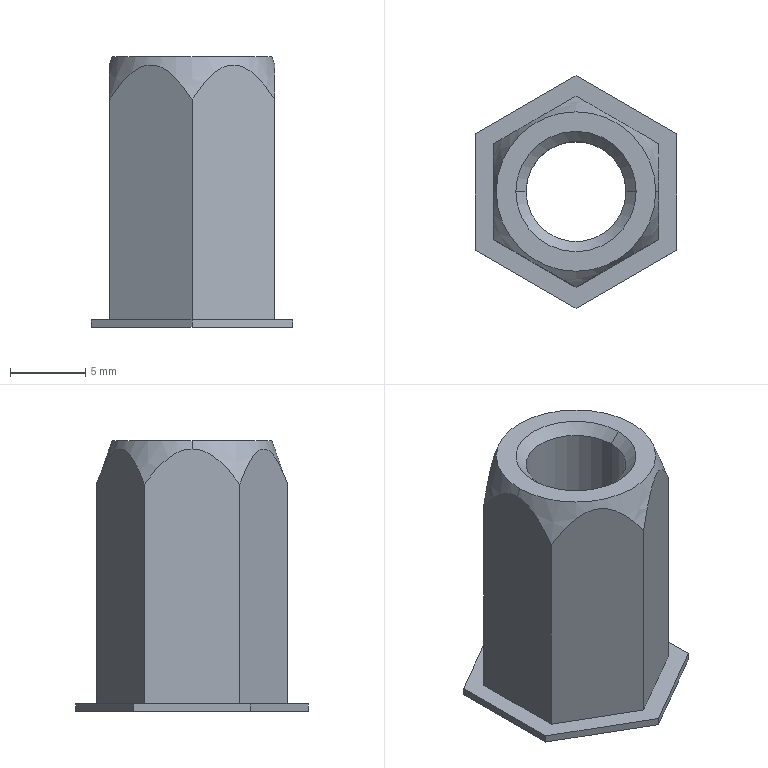Part | NX | features solid 2 | 1 solid | 25 faces | box 13.4 x 15.473 x 18 mm | volume 806.547 mm3 | plane 15 | cone 6 | cylinder 4 | commonest cylinder face diameters 6.647 x2 10.6 x2
STEP:
#1=CARTESIAN_POINT('',(-279.3,516.028,-1067.5));
#2=VERTEX_POINT('',#1);
#3=CARTESIAN_POINT('',(-286.,519.896,-1067.5));
#4=VERTEX_POINT('',#3);
#5=CARTESIAN_POINT('',(-279.3,516.028,-1067.5));
#6=DIRECTION('',(-0.866,0.5,0.));
#7=VECTOR('',#6,1000.);
#8=LINE('',#5,#7);
#9=EDGE_CURVE('',#2,#4,#8,.T.);
#10=ORIENTED_EDGE('',*,*,#9,.F.);
#11=CARTESIAN_POINT('',(-279.3,508.292,-1067.5));
#12=VERTEX_POINT('',#11);
#13=CARTESIAN_POINT('',(-279.3,508.292,-1067.5));
#14=DIRECTION('',(0.,1.,0.));
#15=VECTOR('',#14,1000.);
#16=LINE('',#13,#15);
#17=EDGE_CURVE('',#12,#2,#16,.T.);
#18=ORIENTED_EDGE('',*,*,#17,.F.);
#19=CARTESIAN_POINT('',(-286.,504.424,-1067.5));
#20=VERTEX_POINT('',#19);
#21=CARTESIAN_POINT('',(-286.,504.424,-1067.5));
#22=DIRECTION('',(0.866,0.5,0.));
#23=VECTOR('',#22,1000.);
#24=LINE('',#21,#23);
#25=EDGE_CURVE('',#20,#12,#24,.T.);
#26=ORIENTED_EDGE('',*,*,#25,.F.);
#27=CARTESIAN_POINT('',(-292.7,508.292,-1067.5));
#28=VERTEX_POINT('',#27);
#29=CARTESIAN_POINT('',(-292.7,508.292,-1067.5));
#30=DIRECTION('',(0.866,-0.5,0.));
#31=VECTOR('',#30,1000.);
#32=LINE('',#29,#31);
#33=EDGE_CURVE('',#28,#20,#32,.T.);
#34=ORIENTED_EDGE('',*,*,#33,.F.);
#35=CARTESIAN_POINT('',(-292.7,516.028,-1067.5));
#36=VERTEX_POINT('',#35);
#37=CARTESIAN_POINT('',(-292.7,516.028,-1067.5));
#38=DIRECTION('',(0.,-1.,0.));
#39=VECTOR('',#38,1000.);
#40=LINE('',#37,#39);
#41=EDGE_CURVE('',#36,#28,#40,.T.);
#42=ORIENTED_EDGE('',*,*,#41,.F.);
#43=CARTESIAN_POINT('',(-286.,519.896,-1067.5));
#44=DIRECTION('',(-0.866,-0.5,0.));
#45=VECTOR('',#44,1000.);
#46=LINE('',#43,#45);
#47=EDGE_CURVE('',#4,#36,#46,.T.);
#48=ORIENTED_EDGE('',*,*,#47,.F.);
#49=EDGE_LOOP('',(#10,#18,#26,#34,#42,#48));
#50=FACE_BOUND('',#49,.T.);
#51=CARTESIAN_POINT('',(-291.3,512.16,-1067.5));
#52=VERTEX_POINT('',#51);
#53=CARTESIAN_POINT('',(-280.7,512.16,-1067.5));
#54=VERTEX_POINT('',#53);
#55=CARTESIAN_POINT('',(-286.,512.16,-1067.5));
#56=DIRECTION('',(0.,0.,-1.));
#57=DIRECTION('',(-1.,0.,0.));
#58=AXIS2_PLACEMENT_3D('',#55,#56,#57);
#59=CIRCLE('',#58,5.3);
#60=EDGE_CURVE('',#52,#54,#59,.T.);
#61=ORIENTED_EDGE('',*,*,#60,.F.);
#62=CARTESIAN_POINT('',(-286.,512.16,-1067.5));
#63=DIRECTION('',(0.,0.,-1.));
#64=DIRECTION('',(1.,0.,0.));
#65=AXIS2_PLACEMENT_3D('',#62,#63,#64);
#66=CIRCLE('',#65,5.3);
#67=EDGE_CURVE('',#54,#52,#66,.T.);
#68=ORIENTED_EDGE('',*,*,#67,.F.);
#69=EDGE_LOOP('',(#61,#68));
#70=FACE_BOUND('',#69,.T.);
#71=CARTESIAN_POINT('',(-286.,512.16,-1067.5));
#72=DIRECTION('',(0.,0.,1.));
#73=DIRECTION('',(-1.,0.,0.));
#74=AXIS2_PLACEMENT_3D('',#71,#72,#73);
#75=PLANE('',#74);
#76=ADVANCED_FACE('',(#50,#70),#75,.F.);
#77=CARTESIAN_POINT('',(-292.7,516.028,-1067.));
#78=VERTEX_POINT('',#77);
#79=CARTESIAN_POINT('',(-292.7,516.028,-1067.5));
#80=DIRECTION('',(0.,0.,1.));
#81=VECTOR('',#80,1000.);
#82=LINE('',#79,#81);
#83=EDGE_CURVE('',#36,#78,#82,.T.);
#84=ORIENTED_EDGE('',*,*,#83,.T.);
#85=CARTESIAN_POINT('',(-286.,519.896,-1067.));
#86=VERTEX_POINT('',#85);
#87=CARTESIAN_POINT('',(-292.7,516.028,-1067.));
#88=DIRECTION('',(0.866,0.5,0.));
#89=VECTOR('',#88,1000.);
#90=LINE('',#87,#89);
#91=EDGE_CURVE('',#78,#86,#90,.T.);
#92=ORIENTED_EDGE('',*,*,#91,.T.);
#93=CARTESIAN_POINT('',(-286.,519.896,-1067.5));
#94=DIRECTION('',(0.,0.,1.));
#95=VECTOR('',#94,1000.);
#96=LINE('',#93,#95);
#97=EDGE_CURVE('',#4,#86,#96,.T.);
#98=ORIENTED_EDGE('',*,*,#97,.F.);
#99=ORIENTED_EDGE('',*,*,#47,.T.);
#100=EDGE_LOOP('',(#84,#92,#98,#99));
#101=FACE_BOUND('',#100,.T.);
#102=CARTESIAN_POINT('',(-286.,519.896,-1067.5));
#103=DIRECTION('',(-0.5,0.866,0.));
#104=DIRECTION('',(0.866,0.5,0.));
#105=AXIS2_PLACEMENT_3D('',#102,#103,#104);
#106=PLANE('',#105);
#107=ADVANCED_FACE('',(#101),#106,.T.);
#108=ORIENTED_EDGE('',*,*,#97,.T.);
#109=CARTESIAN_POINT('',(-279.3,516.028,-1067.));
#110=VERTEX_POINT('',#109);
#111=CARTESIAN_POINT('',(-286.,519.896,-1067.));
#112=DIRECTION('',(0.866,-0.5,0.));
#113=VECTOR('',#112,1000.);
#114=LINE('',#111,#113);
#115=EDGE_CURVE('',#86,#110,#114,.T.);
#116=ORIENTED_EDGE('',*,*,#115,.T.);
#117=CARTESIAN_POINT('',(-279.3,516.028,-1067.5));
#118=DIRECTION('',(0.,0.,1.));
#119=VECTOR('',#118,1000.);
#120=LINE('',#117,#119);
#121=EDGE_CURVE('',#2,#110,#120,.T.);
#122=ORIENTED_EDGE('',*,*,#121,.F.);
#123=ORIENTED_EDGE('',*,*,#9,.T.);
#124=EDGE_LOOP('',(#108,#116,#122,#123));
#125=FACE_BOUND('',#124,.T.);
#126=CARTESIAN_POINT('',(-279.3,516.028,-1067.5));
#127=DIRECTION('',(0.5,0.866,0.));
#128=DIRECTION('',(0.866,-0.5,0.));
#129=AXIS2_PLACEMENT_3D('',#126,#127,#128);
#130=PLANE('',#129);
#131=ADVANCED_FACE('',(#125),#130,.T.);
#132=ORIENTED_EDGE('',*,*,#121,.T.);
#133=CARTESIAN_POINT('',(-279.3,508.292,-1067.));
#134=VERTEX_POINT('',#133);
#135=CARTESIAN_POINT('',(-279.3,516.028,-1067.));
#136=DIRECTION('',(0.,-1.,0.));
#137=VECTOR('',#136,1000.);
#138=LINE('',#135,#137);
#139=EDGE_CURVE('',#110,#134,#138,.T.);
#140=ORIENTED_EDGE('',*,*,#139,.T.);
#141=CARTESIAN_POINT('',(-279.3,508.292,-1067.5));
#142=DIRECTION('',(0.,0.,1.));
#143=VECTOR('',#142,1000.);
#144=LINE('',#141,#143);
#145=EDGE_CURVE('',#12,#134,#144,.T.);
#146=ORIENTED_EDGE('',*,*,#145,.F.);
#147=ORIENTED_EDGE('',*,*,#17,.T.);
#148=EDGE_LOOP('',(#132,#140,#146,#147));
#149=FACE_BOUND('',#148,.T.);
#150=CARTESIAN_POINT('',(-279.3,508.292,-1067.5));
#151=DIRECTION('',(1.,0.,0.));
#152=DIRECTION('',(0.,-1.,0.));
#153=AXIS2_PLACEMENT_3D('',#150,#151,#152);
#154=PLANE('',#153);
#155=ADVANCED_FACE('',(#149),#154,.T.);
#156=ORIENTED_EDGE('',*,*,#145,.T.);
#157=CARTESIAN_POINT('',(-286.,504.424,-1067.));
#158=VERTEX_POINT('',#157);
#159=CARTESIAN_POINT('',(-279.3,508.292,-1067.));
#160=DIRECTION('',(-0.866,-0.5,0.));
#161=VECTOR('',#160,1000.);
#162=LINE('',#159,#161);
#163=EDGE_CURVE('',#134,#158,#162,.T.);
#164=ORIENTED_EDGE('',*,*,#163,.T.);
#165=CARTESIAN_POINT('',(-286.,504.424,-1067.5));
#166=DIRECTION('',(0.,0.,1.));
#167=VECTOR('',#166,1000.);
#168=LINE('',#165,#167);
#169=EDGE_CURVE('',#20,#158,#168,.T.);
#170=ORIENTED_EDGE('',*,*,#169,.F.);
#171=ORIENTED_EDGE('',*,*,#25,.T.);
#172=EDGE_LOOP('',(#156,#164,#170,#171));
#173=FACE_BOUND('',#172,.T.);
#174=CARTESIAN_POINT('',(-286.,504.424,-1067.5));
#175=DIRECTION('',(0.5,-0.866,0.));
#176=DIRECTION('',(-0.866,-0.5,0.));
#177=AXIS2_PLACEMENT_3D('',#174,#175,#176);
#178=PLANE('',#177);
#179=ADVANCED_FACE('',(#173),#178,.T.);
#180=ORIENTED_EDGE('',*,*,#169,.T.);
#181=CARTESIAN_POINT('',(-292.7,508.292,-1067.));
#182=VERTEX_POINT('',#181);
#183=CARTESIAN_POINT('',(-286.,504.424,-1067.));
#184=DIRECTION('',(-0.866,0.5,0.));
#185=VECTOR('',#184,1000.);
#186=LINE('',#183,#185);
#187=EDGE_CURVE('',#158,#182,#186,.T.);
#188=ORIENTED_EDGE('',*,*,#187,.T.);
#189=CARTESIAN_POINT('',(-292.7,508.292,-1067.5));
#190=DIRECTION('',(0.,0.,1.));
#191=VECTOR('',#190,1000.);
#192=LINE('',#189,#191);
#193=EDGE_CURVE('',#28,#182,#192,.T.);
#194=ORIENTED_EDGE('',*,*,#193,.F.);
#195=ORIENTED_EDGE('',*,*,#33,.T.);
#196=EDGE_LOOP('',(#180,#188,#194,#195));
#197=FACE_BOUND('',#196,.T.);
#198=CARTESIAN_POINT('',(-292.7,508.292,-1067.5));
#199=DIRECTION('',(-0.5,-0.866,0.));
#200=DIRECTION('',(-0.866,0.5,0.));
#201=AXIS2_PLACEMENT_3D('',#198,#199,#200);
#202=PLANE('',#201);
#203=ADVANCED_FACE('',(#197),#202,.T.);
#204=ORIENTED_EDGE('',*,*,#193,.T.);
#205=CARTESIAN_POINT('',(-292.7,508.292,-1067.));
#206=DIRECTION('',(0.,1.,0.));
#207=VECTOR('',#206,1000.);
#208=LINE('',#205,#207);
#209=EDGE_CURVE('',#182,#78,#208,.T.);
#210=ORIENTED_EDGE('',*,*,#209,.T.);
#211=ORIENTED_EDGE('',*,*,#83,.F.);
#212=ORIENTED_EDGE('',*,*,#41,.T.);
#213=EDGE_LOOP('',(#204,#210,#211,#212));
#214=FACE_BOUND('',#213,.T.);
#215=CARTESIAN_POINT('',(-292.7,516.028,-1067.5));
#216=DIRECTION('',(-1.,0.,0.));
#217=DIRECTION('',(0.,1.,0.));
#218=AXIS2_PLACEMENT_3D('',#215,#216,#217);
#219=PLANE('',#218);
#220=ADVANCED_FACE('',(#214),#219,.T.);
#221=ORIENTED_EDGE('',*,*,#187,.F.);
#222=ORIENTED_EDGE('',*,*,#163,.F.);
#223=ORIENTED_EDGE('',*,*,#139,.F.);
#224=ORIENTED_EDGE('',*,*,#115,.F.);
#225=ORIENTED_EDGE('',*,*,#91,.F.);
#226=ORIENTED_EDGE('',*,*,#209,.F.);
#227=EDGE_LOOP('',(#221,#222,#223,#224,#225,#226));
#228=FACE_BOUND('',#227,.T.);
#229=CARTESIAN_POINT('',(-286.,505.809,-1067.));
#230=VERTEX_POINT('',#229);
#231=CARTESIAN_POINT('',(-280.5,508.985,-1067.));
#232=VERTEX_POINT('',#231);
#233=CARTESIAN_POINT('',(-286.,505.809,-1067.));
#234=DIRECTION('',(0.866,0.5,0.));
#235=VECTOR('',#234,1000.);
#236=LINE('',#233,#235);
#237=EDGE_CURVE('',#230,#232,#236,.T.);
#238=ORIENTED_EDGE('',*,*,#237,.F.);
#239=CARTESIAN_POINT('',(-291.5,508.985,-1067.));
#240=VERTEX_POINT('',#239);
#241=CARTESIAN_POINT('',(-291.5,508.985,-1067.));
#242=DIRECTION('',(0.866,-0.5,0.));
#243=VECTOR('',#242,1000.);
#244=LINE('',#241,#243);
#245=EDGE_CURVE('',#240,#230,#244,.T.);
#246=ORIENTED_EDGE('',*,*,#245,.F.);
#247=CARTESIAN_POINT('',(-291.5,515.335,-1067.));
#248=VERTEX_POINT('',#247);
#249=CARTESIAN_POINT('',(-291.5,515.335,-1067.));
#250=DIRECTION('',(0.,-1.,0.));
#251=VECTOR('',#250,1000.);
#252=LINE('',#249,#251);
#253=EDGE_CURVE('',#248,#240,#252,.T.);
#254=ORIENTED_EDGE('',*,*,#253,.F.);
#255=CARTESIAN_POINT('',(-286.,518.511,-1067.));
#256=VERTEX_POINT('',#255);
#257=CARTESIAN_POINT('',(-286.,518.511,-1067.));
#258=DIRECTION('',(-0.866,-0.5,0.));
#259=VECTOR('',#258,1000.);
#260=LINE('',#257,#259);
#261=EDGE_CURVE('',#256,#248,#260,.T.);
#262=ORIENTED_EDGE('',*,*,#261,.F.);
#263=CARTESIAN_POINT('',(-280.5,515.335,-1067.));
#264=VERTEX_POINT('',#263);
#265=CARTESIAN_POINT('',(-280.5,515.335,-1067.));
#266=DIRECTION('',(-0.866,0.5,0.));
#267=VECTOR('',#266,1000.);
#268=LINE('',#265,#267);
#269=EDGE_CURVE('',#264,#256,#268,.T.);
#270=ORIENTED_EDGE('',*,*,#269,.F.);
#271=CARTESIAN_POINT('',(-280.5,508.985,-1067.));
#272=DIRECTION('',(0.,1.,0.));
#273=VECTOR('',#272,1000.);
#274=LINE('',#271,#273);
#275=EDGE_CURVE('',#232,#264,#274,.T.);
#276=ORIENTED_EDGE('',*,*,#275,.F.);
#277=EDGE_LOOP('',(#238,#246,#254,#262,#270,#276));
#278=FACE_BOUND('',#277,.T.);
#279=CARTESIAN_POINT('',(-286.,512.16,-1067.));
#280=DIRECTION('',(0.,0.,-1.));
#281=DIRECTION('',(1.,0.,0.));
#282=AXIS2_PLACEMENT_3D('',#279,#280,#281);
#283=PLANE('',#282);
#284=ADVANCED_FACE('',(#228,#278),#283,.F.);
#285=CARTESIAN_POINT('',(-280.5,508.985,-1052.387));
#286=VERTEX_POINT('',#285);
#287=CARTESIAN_POINT('',(-280.5,508.985,-1067.));
#288=DIRECTION('',(0.,0.,1.));
#289=VECTOR('',#288,1000.);
#290=LINE('',#287,#289);
#291=EDGE_CURVE('',#232,#286,#290,.T.);
#292=ORIENTED_EDGE('',*,*,#291,.F.);
#293=ORIENTED_EDGE('',*,*,#275,.T.);
#294=CARTESIAN_POINT('',(-280.5,515.335,-1052.387));
#295=VERTEX_POINT('',#294);
#296=CARTESIAN_POINT('',(-280.5,515.335,-1067.));
#297=DIRECTION('',(0.,0.,1.));
#298=VECTOR('',#297,1000.);
#299=LINE('',#296,#298);
#300=EDGE_CURVE('',#264,#295,#299,.T.);
#301=ORIENTED_EDGE('',*,*,#300,.T.);
#302=CARTESIAN_POINT('',(-280.5,512.16,-1050.049));
#303=VERTEX_POINT('',#302);
#304=CARTESIAN_POINT('',(-280.5,512.16,-1050.049));
#305=CARTESIAN_POINT('',(-280.5,512.223,-1050.049));
#306=CARTESIAN_POINT('',(-280.5,512.35,-1050.055));
#307=CARTESIAN_POINT('',(-280.5,512.542,-1050.083));
#308=CARTESIAN_POINT('',(-280.5,512.736,-1050.129));
#309=CARTESIAN_POINT('',(-280.5,512.937,-1050.196));
#310=CARTESIAN_POINT('',(-280.5,513.143,-1050.285));
#311=CARTESIAN_POINT('',(-280.5,513.359,-1050.4));
#312=CARTESIAN_POINT('',(-280.5,513.586,-1050.545));
#313=CARTESIAN_POINT('',(-280.5,513.827,-1050.724));
#314=CARTESIAN_POINT('',(-280.5,514.085,-1050.944));
#315=CARTESIAN_POINT('',(-280.5,514.364,-1051.212));
#316=CARTESIAN_POINT('',(-280.5,514.664,-1051.536));
#317=CARTESIAN_POINT('',(-280.5,514.986,-1051.921));
#318=CARTESIAN_POINT('',(-280.5,515.217,-1052.224));
#319=CARTESIAN_POINT('',(-280.5,515.335,-1052.387));
#320=B_SPLINE_CURVE_WITH_KNOTS('',3,(#304,#305,#306,#307,#308,#309,#310,#311,#312,#313,#314,#315,#316,#317,#318,#319),.UNSPECIFIED.,.F.,.F.,(4,1,1,1,1,1,1,1,1,1,1,1,1,4),(0.,0.07692,0.1538,0.2308,0.3077,0.3846,0.4615,0.5385,0.6154,0.6923,0.7692,0.8462,0.9231,1.),.QUASI_UNIFORM_KNOTS.);
#321=EDGE_CURVE('',#303,#295,#320,.T.);
#322=ORIENTED_EDGE('',*,*,#321,.F.);
#323=CARTESIAN_POINT('',(-280.5,512.16,-1050.049));
#324=CARTESIAN_POINT('',(-280.5,512.097,-1050.049));
#325=CARTESIAN_POINT('',(-280.5,511.97,-1050.055));
#326=CARTESIAN_POINT('',(-280.5,511.779,-1050.083));
#327=CARTESIAN_POINT('',(-280.5,511.584,-1050.129));
#328=CARTESIAN_POINT('',(-280.5,511.384,-1050.196));
#329=CARTESIAN_POINT('',(-280.5,511.178,-1050.285));
#330=CARTESIAN_POINT('',(-280.5,510.962,-1050.4));
#331=CARTESIAN_POINT('',(-280.5,510.734,-1050.545));
#332=CARTESIAN_POINT('',(-280.5,510.494,-1050.723));
#333=CARTESIAN_POINT('',(-280.5,510.235,-1050.943));
#334=CARTESIAN_POINT('',(-280.5,509.956,-1051.212));
#335=CARTESIAN_POINT('',(-280.5,509.656,-1051.536));
#336=CARTESIAN_POINT('',(-280.5,509.334,-1051.921));
#337=CARTESIAN_POINT('',(-280.5,509.103,-1052.224));
#338=CARTESIAN_POINT('',(-280.5,508.985,-1052.387));
#339=B_SPLINE_CURVE_WITH_KNOTS('',3,(#323,#324,#325,#326,#327,#328,#329,#330,#331,#332,#333,#334,#335,#336,#337,#338),.UNSPECIFIED.,.F.,.F.,(4,1,1,1,1,1,1,1,1,1,1,1,1,4),(0.,0.07692,0.1538,0.2308,0.3077,0.3846,0.4615,0.5385,0.6154,0.6923,0.7692,0.8462,0.9231,1.),.QUASI_UNIFORM_KNOTS.);
#340=EDGE_CURVE('',#303,#286,#339,.T.);
#341=ORIENTED_EDGE('',*,*,#340,.T.);
#342=EDGE_LOOP('',(#292,#293,#301,#322,#341));
#343=FACE_BOUND('',#342,.T.);
#344=CARTESIAN_POINT('',(-280.5,508.985,-1067.));
#345=DIRECTION('',(-1.,0.,0.));
#346=DIRECTION('',(0.,-1.,0.));
#347=AXIS2_PLACEMENT_3D('',#344,#345,#346);
#348=PLANE('',#347);
#349=ADVANCED_FACE('',(#343),#348,.F.);
#350=CARTESIAN_POINT('',(-280.7,512.16,-1049.5));
#351=VERTEX_POINT('',#350);
#352=CARTESIAN_POINT('',(-280.7,512.16,-1049.5));
#353=DIRECTION('',(0.342,0.,-0.9397));
#354=VECTOR('',#353,1000.);
#355=LINE('',#352,#354);
#356=EDGE_CURVE('',#303,#351,#355,.F.);
#357=ORIENTED_EDGE('',*,*,#356,.T.);
#358=CARTESIAN_POINT('',(-291.3,512.16,-1049.5));
#359=VERTEX_POINT('',#358);
#360=CARTESIAN_POINT('',(-286.,512.16,-1049.5));
#361=DIRECTION('',(0.,0.,-1.));
#362=DIRECTION('',(1.,0.,0.));
#363=AXIS2_PLACEMENT_3D('',#360,#361,#362);
#364=CIRCLE('',#363,5.3);
#365=EDGE_CURVE('',#351,#359,#364,.T.);
#366=ORIENTED_EDGE('',*,*,#365,.T.);
#367=CARTESIAN_POINT('',(-291.5,512.16,-1050.049));
#368=VERTEX_POINT('',#367);
#369=CARTESIAN_POINT('',(-291.3,512.16,-1049.5));
#370=DIRECTION('',(-0.342,0.,-0.9397));
#371=VECTOR('',#370,1000.);
#372=LINE('',#369,#371);
#373=EDGE_CURVE('',#359,#368,#372,.T.);
#374=ORIENTED_EDGE('',*,*,#373,.T.);
#375=CARTESIAN_POINT('',(-291.5,508.985,-1052.387));
#376=VERTEX_POINT('',#375);
#377=CARTESIAN_POINT('',(-291.5,512.16,-1050.049));
#378=CARTESIAN_POINT('',(-291.5,512.097,-1050.049));
#379=CARTESIAN_POINT('',(-291.5,511.97,-1050.055));
#380=CARTESIAN_POINT('',(-291.5,511.778,-1050.083));
#381=CARTESIAN_POINT('',(-291.5,511.584,-1050.129));
#382=CARTESIAN_POINT('',(-291.5,511.383,-1050.196));
#383=CARTESIAN_POINT('',(-291.5,511.177,-1050.285));
#384=CARTESIAN_POINT('',(-291.5,510.961,-1050.4));
#385=CARTESIAN_POINT('',(-291.5,510.734,-1050.545));
#386=CARTESIAN_POINT('',(-291.5,510.493,-1050.724));
#387=CARTESIAN_POINT('',(-291.5,510.235,-1050.944));
#388=CARTESIAN_POINT('',(-291.5,509.956,-1051.212));
#389=CARTESIAN_POINT('',(-291.5,509.656,-1051.536));
#390=CARTESIAN_POINT('',(-291.5,509.334,-1051.921));
#391=CARTESIAN_POINT('',(-291.5,509.103,-1052.224));
#392=CARTESIAN_POINT('',(-291.5,508.985,-1052.387));
#393=B_SPLINE_CURVE_WITH_KNOTS('',3,(#377,#378,#379,#380,#381,#382,#383,#384,#385,#386,#387,#388,#389,#390,#391,#392),.UNSPECIFIED.,.F.,.F.,(4,1,1,1,1,1,1,1,1,1,1,1,1,4),(0.,0.07692,0.1538,0.2308,0.3077,0.3846,0.4615,0.5385,0.6154,0.6923,0.7692,0.8462,0.9231,1.),.QUASI_UNIFORM_KNOTS.);
#394=EDGE_CURVE('',#368,#376,#393,.T.);
#395=ORIENTED_EDGE('',*,*,#394,.T.);
#396=CARTESIAN_POINT('',(-286.,505.809,-1052.387));
#397=VERTEX_POINT('',#396);
#398=CARTESIAN_POINT('',(-291.5,508.985,-1052.387));
#399=CARTESIAN_POINT('',(-291.393,508.923,-1052.217));
#400=CARTESIAN_POINT('',(-291.185,508.803,-1051.903));
#401=CARTESIAN_POINT('',(-290.896,508.636,-1051.506));
#402=CARTESIAN_POINT('',(-290.627,508.481,-1051.175));
#403=CARTESIAN_POINT('',(-290.377,508.336,-1050.902));
#404=CARTESIAN_POINT('',(-290.146,508.203,-1050.68));
#405=CARTESIAN_POINT('',(-289.931,508.079,-1050.503));
#406=CARTESIAN_POINT('',(-289.729,507.962,-1050.361));
#407=CARTESIAN_POINT('',(-289.538,507.852,-1050.251));
#408=CARTESIAN_POINT('',(-289.355,507.746,-1050.167));
#409=CARTESIAN_POINT('',(-289.179,507.645,-1050.107));
#410=CARTESIAN_POINT('',(-289.007,507.545,-1050.068));
#411=CARTESIAN_POINT('',(-288.837,507.447,-1050.049));
#412=CARTESIAN_POINT('',(-288.669,507.35,-1050.049));
#413=CARTESIAN_POINT('',(-288.499,507.252,-1050.067));
#414=CARTESIAN_POINT('',(-288.328,507.153,-1050.105));
#415=CARTESIAN_POINT('',(-288.152,507.052,-1050.165));
#416=CARTESIAN_POINT('',(-287.97,506.947,-1050.247));
#417=CARTESIAN_POINT('',(-287.78,506.837,-1050.356));
#418=CARTESIAN_POINT('',(-287.578,506.72,-1050.496));
#419=CARTESIAN_POINT('',(-287.363,506.596,-1050.672));
#420=CARTESIAN_POINT('',(-287.131,506.462,-1050.893));
#421=CARTESIAN_POINT('',(-286.88,506.317,-1051.166));
#422=CARTESIAN_POINT('',(-286.609,506.161,-1051.5));
#423=CARTESIAN_POINT('',(-286.317,505.992,-1051.899));
#424=CARTESIAN_POINT('',(-286.108,505.871,-1052.216));
#425=CARTESIAN_POINT('',(-286.,505.809,-1052.387));
#426=B_SPLINE_CURVE_WITH_KNOTS('',3,(#398,#399,#400,#401,#402,#403,#404,#405,#406,#407,#408,#409,#410,#411,#412,#413,#414,#415,#416,#417,#418,#419,#420,#421,#422,#423,#424,#425),.UNSPECIFIED.,.F.,.F.,(4,1,1,1,1,1,1,1,1,1,1,1,1,1,1,1,1,1,1,1,1,1,1,1,1,4),(0.,0.04,0.08,0.12,0.16,0.2,0.24,0.28,0.32,0.36,0.4,0.44,0.48,0.52,0.56,0.6,0.64,0.68,0.72,0.76,0.8,0.84,0.88,0.92,0.96,1.),.QUASI_UNIFORM_KNOTS.);
#427=EDGE_CURVE('',#376,#397,#426,.T.);
#428=ORIENTED_EDGE('',*,*,#427,.T.);
#429=CARTESIAN_POINT('',(-286.,505.809,-1052.387));
#430=CARTESIAN_POINT('',(-285.893,505.871,-1052.217));
#431=CARTESIAN_POINT('',(-285.685,505.991,-1051.903));
#432=CARTESIAN_POINT('',(-285.396,506.158,-1051.506));
#433=CARTESIAN_POINT('',(-285.127,506.313,-1051.175));
#434=CARTESIAN_POINT('',(-284.877,506.457,-1050.902));
#435=CARTESIAN_POINT('',(-284.646,506.591,-1050.68));
#436=CARTESIAN_POINT('',(-284.431,506.715,-1050.503));
#437=CARTESIAN_POINT('',(-284.229,506.832,-1050.361));
#438=CARTESIAN_POINT('',(-284.038,506.942,-1050.251));
#439=CARTESIAN_POINT('',(-283.855,507.048,-1050.167));
#440=CARTESIAN_POINT('',(-283.679,507.149,-1050.107));
#441=CARTESIAN_POINT('',(-283.507,507.249,-1050.068));
#442=CARTESIAN_POINT('',(-283.337,507.347,-1050.049));
#443=CARTESIAN_POINT('',(-283.169,507.444,-1050.049));
#444=CARTESIAN_POINT('',(-282.999,507.542,-1050.067));
#445=CARTESIAN_POINT('',(-282.828,507.64,-1050.105));
#446=CARTESIAN_POINT('',(-282.652,507.742,-1050.165));
#447=CARTESIAN_POINT('',(-282.47,507.847,-1050.247));
#448=CARTESIAN_POINT('',(-282.28,507.957,-1050.356));
#449=CARTESIAN_POINT('',(-282.078,508.073,-1050.496));
#450=CARTESIAN_POINT('',(-281.863,508.198,-1050.672));
#451=CARTESIAN_POINT('',(-281.631,508.332,-1050.893));
#452=CARTESIAN_POINT('',(-281.38,508.477,-1051.166));
#453=CARTESIAN_POINT('',(-281.109,508.633,-1051.5));
#454=CARTESIAN_POINT('',(-280.817,508.801,-1051.899));
#455=CARTESIAN_POINT('',(-280.608,508.922,-1052.216));
#456=CARTESIAN_POINT('',(-280.5,508.985,-1052.387));
#457=B_SPLINE_CURVE_WITH_KNOTS('',3,(#429,#430,#431,#432,#433,#434,#435,#436,#437,#438,#439,#440,#441,#442,#443,#444,#445,#446,#447,#448,#449,#450,#451,#452,#453,#454,#455,#456),.UNSPECIFIED.,.F.,.F.,(4,1,1,1,1,1,1,1,1,1,1,1,1,1,1,1,1,1,1,1,1,1,1,1,1,4),(0.,0.04,0.08,0.12,0.16,0.2,0.24,0.28,0.32,0.36,0.4,0.44,0.48,0.52,0.56,0.6,0.64,0.68,0.72,0.76,0.8,0.84,0.88,0.92,0.96,1.),.QUASI_UNIFORM_KNOTS.);
#458=EDGE_CURVE('',#397,#286,#457,.T.);
#459=ORIENTED_EDGE('',*,*,#458,.T.);
#460=ORIENTED_EDGE('',*,*,#340,.F.);
#461=EDGE_LOOP('',(#357,#366,#374,#395,#428,#459,#460));
#462=FACE_BOUND('',#461,.T.);
#463=CARTESIAN_POINT('',(-286.,512.16,-1050.944));
#464=DIRECTION('',(0.,0.,-1.));
#465=DIRECTION('',(1.,0.,0.));
#466=AXIS2_PLACEMENT_3D('',#463,#464,#465);
#467=CONICAL_SURFACE('',#466,5.825,0.3491);
#468=ADVANCED_FACE('',(#462),#467,.T.);
#469=CARTESIAN_POINT('',(-286.,505.809,-1067.));
#470=DIRECTION('',(0.,0.,1.));
#471=VECTOR('',#470,1000.);
#472=LINE('',#469,#471);
#473=EDGE_CURVE('',#230,#397,#472,.T.);
#474=ORIENTED_EDGE('',*,*,#473,.F.);
#475=ORIENTED_EDGE('',*,*,#237,.T.);
#476=ORIENTED_EDGE('',*,*,#291,.T.);
#477=ORIENTED_EDGE('',*,*,#458,.F.);
#478=EDGE_LOOP('',(#474,#475,#476,#477));
#479=FACE_BOUND('',#478,.T.);
#480=CARTESIAN_POINT('',(-286.,505.809,-1067.));
#481=DIRECTION('',(-0.5,0.866,0.));
#482=DIRECTION('',(-0.866,-0.5,0.));
#483=AXIS2_PLACEMENT_3D('',#480,#481,#482);
#484=PLANE('',#483);
#485=ADVANCED_FACE('',(#479),#484,.F.);
#486=CARTESIAN_POINT('',(-291.5,508.985,-1067.));
#487=DIRECTION('',(0.,0.,1.));
#488=VECTOR('',#487,1000.);
#489=LINE('',#486,#488);
#490=EDGE_CURVE('',#240,#376,#489,.T.);
#491=ORIENTED_EDGE('',*,*,#490,.F.);
#492=ORIENTED_EDGE('',*,*,#245,.T.);
#493=ORIENTED_EDGE('',*,*,#473,.T.);
#494=ORIENTED_EDGE('',*,*,#427,.F.);
#495=EDGE_LOOP('',(#491,#492,#493,#494));
#496=FACE_BOUND('',#495,.T.);
#497=CARTESIAN_POINT('',(-291.5,508.985,-1067.));
#498=DIRECTION('',(0.5,0.866,0.));
#499=DIRECTION('',(-0.866,0.5,0.));
#500=AXIS2_PLACEMENT_3D('',#497,#498,#499);
#501=PLANE('',#500);
#502=ADVANCED_FACE('',(#496),#501,.F.);
#503=CARTESIAN_POINT('',(-291.5,515.335,-1052.387));
#504=VERTEX_POINT('',#503);
#505=CARTESIAN_POINT('',(-291.5,512.16,-1050.049));
#506=CARTESIAN_POINT('',(-291.5,512.223,-1050.049));
#507=CARTESIAN_POINT('',(-291.5,512.35,-1050.055));
#508=CARTESIAN_POINT('',(-291.5,512.541,-1050.083));
#509=CARTESIAN_POINT('',(-291.5,512.736,-1050.129));
#510=CARTESIAN_POINT('',(-291.5,512.936,-1050.196));
#511=CARTESIAN_POINT('',(-291.5,513.142,-1050.285));
#512=CARTESIAN_POINT('',(-291.5,513.358,-1050.4));
#513=CARTESIAN_POINT('',(-291.5,513.586,-1050.545));
#514=CARTESIAN_POINT('',(-291.5,513.826,-1050.723));
#515=CARTESIAN_POINT('',(-291.5,514.085,-1050.943));
#516=CARTESIAN_POINT('',(-291.5,514.364,-1051.212));
#517=CARTESIAN_POINT('',(-291.5,514.664,-1051.536));
#518=CARTESIAN_POINT('',(-291.5,514.986,-1051.921));
#519=CARTESIAN_POINT('',(-291.5,515.217,-1052.224));
#520=CARTESIAN_POINT('',(-291.5,515.335,-1052.387));
#521=B_SPLINE_CURVE_WITH_KNOTS('',3,(#505,#506,#507,#508,#509,#510,#511,#512,#513,#514,#515,#516,#517,#518,#519,#520),.UNSPECIFIED.,.F.,.F.,(4,1,1,1,1,1,1,1,1,1,1,1,1,4),(0.,0.07692,0.1538,0.2308,0.3077,0.3846,0.4615,0.5385,0.6154,0.6923,0.7692,0.8462,0.9231,1.),.QUASI_UNIFORM_KNOTS.);
#522=EDGE_CURVE('',#368,#504,#521,.T.);
#523=ORIENTED_EDGE('',*,*,#522,.T.);
#524=CARTESIAN_POINT('',(-291.5,515.335,-1067.));
#525=DIRECTION('',(0.,0.,1.));
#526=VECTOR('',#525,1000.);
#527=LINE('',#524,#526);
#528=EDGE_CURVE('',#248,#504,#527,.T.);
#529=ORIENTED_EDGE('',*,*,#528,.F.);
#530=ORIENTED_EDGE('',*,*,#253,.T.);
#531=ORIENTED_EDGE('',*,*,#490,.T.);
#532=ORIENTED_EDGE('',*,*,#394,.F.);
#533=EDGE_LOOP('',(#523,#529,#530,#531,#532));
#534=FACE_BOUND('',#533,.T.);
#535=CARTESIAN_POINT('',(-291.5,515.335,-1067.));
#536=DIRECTION('',(1.,0.,0.));
#537=DIRECTION('',(0.,1.,0.));
#538=AXIS2_PLACEMENT_3D('',#535,#536,#537);
#539=PLANE('',#538);
#540=ADVANCED_FACE('',(#534),#539,.F.);
#541=CARTESIAN_POINT('',(-286.,518.511,-1052.387));
#542=VERTEX_POINT('',#541);
#543=CARTESIAN_POINT('',(-286.,518.511,-1067.));
#544=DIRECTION('',(0.,0.,1.));
#545=VECTOR('',#544,1000.);
#546=LINE('',#543,#545);
#547=EDGE_CURVE('',#256,#542,#546,.T.);
#548=ORIENTED_EDGE('',*,*,#547,.F.);
#549=ORIENTED_EDGE('',*,*,#261,.T.);
#550=ORIENTED_EDGE('',*,*,#528,.T.);
#551=CARTESIAN_POINT('',(-286.,518.511,-1052.387));
#552=CARTESIAN_POINT('',(-286.107,518.449,-1052.217));
#553=CARTESIAN_POINT('',(-286.315,518.329,-1051.903));
#554=CARTESIAN_POINT('',(-286.604,518.162,-1051.506));
#555=CARTESIAN_POINT('',(-286.873,518.007,-1051.175));
#556=CARTESIAN_POINT('',(-287.123,517.863,-1050.902));
#557=CARTESIAN_POINT('',(-287.354,517.729,-1050.68));
#558=CARTESIAN_POINT('',(-287.569,517.605,-1050.503));
#559=CARTESIAN_POINT('',(-287.771,517.488,-1050.361));
#560=CARTESIAN_POINT('',(-287.962,517.378,-1050.251));
#561=CARTESIAN_POINT('',(-288.145,517.272,-1050.167));
#562=CARTESIAN_POINT('',(-288.321,517.171,-1050.107));
#563=CARTESIAN_POINT('',(-288.493,517.071,-1050.068));
#564=CARTESIAN_POINT('',(-288.663,516.973,-1050.049));
#565=CARTESIAN_POINT('',(-288.831,516.876,-1050.049));
#566=CARTESIAN_POINT('',(-289.001,516.778,-1050.067));
#567=CARTESIAN_POINT('',(-289.172,516.68,-1050.105));
#568=CARTESIAN_POINT('',(-289.348,516.578,-1050.165));
#569=CARTESIAN_POINT('',(-289.53,516.473,-1050.247));
#570=CARTESIAN_POINT('',(-289.72,516.363,-1050.356));
#571=CARTESIAN_POINT('',(-289.922,516.247,-1050.496));
#572=CARTESIAN_POINT('',(-290.137,516.122,-1050.672));
#573=CARTESIAN_POINT('',(-290.369,515.988,-1050.893));
#574=CARTESIAN_POINT('',(-290.62,515.843,-1051.166));
#575=CARTESIAN_POINT('',(-290.891,515.687,-1051.5));
#576=CARTESIAN_POINT('',(-291.183,515.519,-1051.899));
#577=CARTESIAN_POINT('',(-291.392,515.398,-1052.216));
#578=CARTESIAN_POINT('',(-291.5,515.335,-1052.387));
#579=B_SPLINE_CURVE_WITH_KNOTS('',3,(#551,#552,#553,#554,#555,#556,#557,#558,#559,#560,#561,#562,#563,#564,#565,#566,#567,#568,#569,#570,#571,#572,#573,#574,#575,#576,#577,#578),.UNSPECIFIED.,.F.,.F.,(4,1,1,1,1,1,1,1,1,1,1,1,1,1,1,1,1,1,1,1,1,1,1,1,1,4),(0.,0.04,0.08,0.12,0.16,0.2,0.24,0.28,0.32,0.36,0.4,0.44,0.48,0.52,0.56,0.6,0.64,0.68,0.72,0.76,0.8,0.84,0.88,0.92,0.96,1.),.QUASI_UNIFORM_KNOTS.);
#580=EDGE_CURVE('',#542,#504,#579,.T.);
#581=ORIENTED_EDGE('',*,*,#580,.F.);
#582=EDGE_LOOP('',(#548,#549,#550,#581));
#583=FACE_BOUND('',#582,.T.);
#584=CARTESIAN_POINT('',(-286.,518.511,-1067.));
#585=DIRECTION('',(0.5,-0.866,0.));
#586=DIRECTION('',(0.866,0.5,0.));
#587=AXIS2_PLACEMENT_3D('',#584,#585,#586);
#588=PLANE('',#587);
#589=ADVANCED_FACE('',(#583),#588,.F.);
#590=CARTESIAN_POINT('',(-280.5,515.335,-1052.387));
#591=CARTESIAN_POINT('',(-280.607,515.397,-1052.217));
#592=CARTESIAN_POINT('',(-280.815,515.517,-1051.903));
#593=CARTESIAN_POINT('',(-281.104,515.684,-1051.506));
#594=CARTESIAN_POINT('',(-281.373,515.839,-1051.175));
#595=CARTESIAN_POINT('',(-281.623,515.984,-1050.902));
#596=CARTESIAN_POINT('',(-281.854,516.117,-1050.68));
#597=CARTESIAN_POINT('',(-282.069,516.241,-1050.503));
#598=CARTESIAN_POINT('',(-282.271,516.358,-1050.361));
#599=CARTESIAN_POINT('',(-282.462,516.468,-1050.251));
#600=CARTESIAN_POINT('',(-282.645,516.574,-1050.167));
#601=CARTESIAN_POINT('',(-282.821,516.675,-1050.107));
#602=CARTESIAN_POINT('',(-282.993,516.775,-1050.068));
#603=CARTESIAN_POINT('',(-283.163,516.873,-1050.049));
#604=CARTESIAN_POINT('',(-283.331,516.97,-1050.049));
#605=CARTESIAN_POINT('',(-283.501,517.068,-1050.067));
#606=CARTESIAN_POINT('',(-283.672,517.167,-1050.105));
#607=CARTESIAN_POINT('',(-283.848,517.268,-1050.165));
#608=CARTESIAN_POINT('',(-284.03,517.373,-1050.247));
#609=CARTESIAN_POINT('',(-284.22,517.483,-1050.356));
#610=CARTESIAN_POINT('',(-284.422,517.6,-1050.496));
#611=CARTESIAN_POINT('',(-284.637,517.724,-1050.672));
#612=CARTESIAN_POINT('',(-284.869,517.858,-1050.893));
#613=CARTESIAN_POINT('',(-285.12,518.003,-1051.166));
#614=CARTESIAN_POINT('',(-285.391,518.159,-1051.5));
#615=CARTESIAN_POINT('',(-285.683,518.328,-1051.899));
#616=CARTESIAN_POINT('',(-285.892,518.449,-1052.216));
#617=CARTESIAN_POINT('',(-286.,518.511,-1052.387));
#618=B_SPLINE_CURVE_WITH_KNOTS('',3,(#590,#591,#592,#593,#594,#595,#596,#597,#598,#599,#600,#601,#602,#603,#604,#605,#606,#607,#608,#609,#610,#611,#612,#613,#614,#615,#616,#617),.UNSPECIFIED.,.F.,.F.,(4,1,1,1,1,1,1,1,1,1,1,1,1,1,1,1,1,1,1,1,1,1,1,1,1,4),(0.,0.04,0.08,0.12,0.16,0.2,0.24,0.28,0.32,0.36,0.4,0.44,0.48,0.52,0.56,0.6,0.64,0.68,0.72,0.76,0.8,0.84,0.88,0.92,0.96,1.),.QUASI_UNIFORM_KNOTS.);
#619=EDGE_CURVE('',#295,#542,#618,.T.);
#620=ORIENTED_EDGE('',*,*,#619,.T.);
#621=ORIENTED_EDGE('',*,*,#580,.T.);
#622=ORIENTED_EDGE('',*,*,#522,.F.);
#623=ORIENTED_EDGE('',*,*,#373,.F.);
#624=CARTESIAN_POINT('',(-286.,512.16,-1049.5));
#625=DIRECTION('',(0.,0.,-1.));
#626=DIRECTION('',(-1.,0.,0.));
#627=AXIS2_PLACEMENT_3D('',#624,#625,#626);
#628=CIRCLE('',#627,5.3);
#629=EDGE_CURVE('',#359,#351,#628,.T.);
#630=ORIENTED_EDGE('',*,*,#629,.T.);
#631=ORIENTED_EDGE('',*,*,#356,.F.);
#632=ORIENTED_EDGE('',*,*,#321,.T.);
#633=EDGE_LOOP('',(#620,#621,#622,#623,#630,#631,#632));
#634=FACE_BOUND('',#633,.T.);
#635=CARTESIAN_POINT('',(-286.,512.16,-1050.944));
#636=DIRECTION('',(0.,0.,-1.));
#637=DIRECTION('',(1.,0.,0.));
#638=AXIS2_PLACEMENT_3D('',#635,#636,#637);
#639=CONICAL_SURFACE('',#638,5.825,0.3491);
#640=ADVANCED_FACE('',(#634),#639,.T.);
#641=ORIENTED_EDGE('',*,*,#629,.F.);
#642=ORIENTED_EDGE('',*,*,#365,.F.);
#643=EDGE_LOOP('',(#641,#642));
#644=FACE_BOUND('',#643,.T.);
#645=CARTESIAN_POINT('',(-290.,512.16,-1049.5));
#646=VERTEX_POINT('',#645);
#647=CARTESIAN_POINT('',(-282.,512.16,-1049.5));
#648=VERTEX_POINT('',#647);
#649=CARTESIAN_POINT('',(-286.,512.16,-1049.5));
#650=DIRECTION('',(0.,0.,1.));
#651=DIRECTION('',(-1.,0.,0.));
#652=AXIS2_PLACEMENT_3D('',#649,#650,#651);
#653=CIRCLE('',#652,4.);
#654=EDGE_CURVE('',#646,#648,#653,.T.);
#655=ORIENTED_EDGE('',*,*,#654,.F.);
#656=CARTESIAN_POINT('',(-286.,512.16,-1049.5));
#657=DIRECTION('',(0.,0.,1.));
#658=DIRECTION('',(1.,0.,0.));
#659=AXIS2_PLACEMENT_3D('',#656,#657,#658);
#660=CIRCLE('',#659,4.);
#661=EDGE_CURVE('',#648,#646,#660,.T.);
#662=ORIENTED_EDGE('',*,*,#661,.F.);
#663=EDGE_LOOP('',(#655,#662));
#664=FACE_BOUND('',#663,.T.);
#665=CARTESIAN_POINT('',(-286.,512.16,-1049.5));
#666=DIRECTION('',(0.,0.,1.));
#667=DIRECTION('',(-1.,0.,0.));
#668=AXIS2_PLACEMENT_3D('',#665,#666,#667);
#669=PLANE('',#668);
#670=ADVANCED_FACE('',(#644,#664),#669,.T.);
#671=CARTESIAN_POINT('',(-282.676,512.16,-1050.177));
#672=VERTEX_POINT('',#671);
#673=CARTESIAN_POINT('',(-289.324,512.16,-1050.177));
#674=VERTEX_POINT('',#673);
#675=CARTESIAN_POINT('',(-286.,512.16,-1050.177));
#676=DIRECTION('',(0.,0.,1.));
#677=DIRECTION('',(1.,0.,0.));
#678=AXIS2_PLACEMENT_3D('',#675,#676,#677);
#679=CIRCLE('',#678,3.324);
#680=EDGE_CURVE('',#672,#674,#679,.T.);
#681=ORIENTED_EDGE('',*,*,#680,.F.);
#682=CARTESIAN_POINT('',(-282.676,512.16,-1050.177));
#683=DIRECTION('',(0.7071,0.,0.7071));
#684=VECTOR('',#683,1000.);
#685=LINE('',#682,#684);
#686=EDGE_CURVE('',#648,#672,#685,.F.);
#687=ORIENTED_EDGE('',*,*,#686,.F.);
#688=ORIENTED_EDGE('',*,*,#661,.T.);
#689=CARTESIAN_POINT('',(-289.324,512.16,-1050.177));
#690=DIRECTION('',(-0.7071,0.,0.7071));
#691=VECTOR('',#690,1000.);
#692=LINE('',#689,#691);
#693=EDGE_CURVE('',#674,#646,#692,.T.);
#694=ORIENTED_EDGE('',*,*,#693,.F.);
#695=EDGE_LOOP('',(#681,#687,#688,#694));
#696=FACE_BOUND('',#695,.T.);
#697=CARTESIAN_POINT('',(-286.,512.16,-1049.838));
#698=DIRECTION('',(0.,0.,1.));
#699=DIRECTION('',(-1.,0.,0.));
#700=AXIS2_PLACEMENT_3D('',#697,#698,#699);
#701=CONICAL_SURFACE('',#700,3.662,0.7854);
#702=ADVANCED_FACE('',(#696),#701,.F.);
#703=ORIENTED_EDGE('',*,*,#654,.T.);
#704=ORIENTED_EDGE('',*,*,#686,.T.);
#705=CARTESIAN_POINT('',(-286.,512.16,-1050.177));
#706=DIRECTION('',(0.,0.,1.));
#707=DIRECTION('',(-1.,0.,0.));
#708=AXIS2_PLACEMENT_3D('',#705,#706,#707);
#709=CIRCLE('',#708,3.324);
#710=EDGE_CURVE('',#674,#672,#709,.T.);
#711=ORIENTED_EDGE('',*,*,#710,.F.);
#712=ORIENTED_EDGE('',*,*,#693,.T.);
#713=EDGE_LOOP('',(#703,#704,#711,#712));
#714=FACE_BOUND('',#713,.T.);
#715=CARTESIAN_POINT('',(-286.,512.16,-1049.838));
#716=DIRECTION('',(0.,0.,1.));
#717=DIRECTION('',(-1.,0.,0.));
#718=AXIS2_PLACEMENT_3D('',#715,#716,#717);
#719=CONICAL_SURFACE('',#718,3.662,0.7854);
#720=ADVANCED_FACE('',(#714),#719,.F.);
#721=ORIENTED_EDGE('',*,*,#710,.T.);
#722=CARTESIAN_POINT('',(-282.676,512.16,-1057.823));
#723=VERTEX_POINT('',#722);
#724=CARTESIAN_POINT('',(-282.676,512.16,-1057.823));
#725=DIRECTION('',(0.,0.,1.));
#726=VECTOR('',#725,1000.);
#727=LINE('',#724,#726);
#728=EDGE_CURVE('',#672,#723,#727,.F.);
#729=ORIENTED_EDGE('',*,*,#728,.T.);
#730=CARTESIAN_POINT('',(-289.324,512.16,-1057.823));
#731=VERTEX_POINT('',#730);
#732=CARTESIAN_POINT('',(-286.,512.16,-1057.823));
#733=DIRECTION('',(0.,0.,-1.));
#734=DIRECTION('',(1.,0.,0.));
#735=AXIS2_PLACEMENT_3D('',#732,#733,#734);
#736=CIRCLE('',#735,3.324);
#737=EDGE_CURVE('',#723,#731,#736,.T.);
#738=ORIENTED_EDGE('',*,*,#737,.T.);
#739=CARTESIAN_POINT('',(-289.324,512.16,-1057.823));
#740=DIRECTION('',(0.,0.,1.));
#741=VECTOR('',#740,1000.);
#742=LINE('',#739,#741);
#743=EDGE_CURVE('',#731,#674,#742,.T.);
#744=ORIENTED_EDGE('',*,*,#743,.T.);
#745=EDGE_LOOP('',(#721,#729,#738,#744));
#746=FACE_BOUND('',#745,.T.);
#747=CARTESIAN_POINT('',(-286.,512.16,-1067.5));
#748=DIRECTION('',(0.,0.,1.));
#749=DIRECTION('',(-1.,0.,0.));
#750=AXIS2_PLACEMENT_3D('',#747,#748,#749);
#751=CYLINDRICAL_SURFACE('',#750,3.324);
#752=ADVANCED_FACE('',(#746),#751,.F.);
#753=CARTESIAN_POINT('',(-286.,512.16,-1057.823));
#754=DIRECTION('',(0.,0.,-1.));
#755=DIRECTION('',(-1.,0.,0.));
#756=AXIS2_PLACEMENT_3D('',#753,#754,#755);
#757=CIRCLE('',#756,3.324);
#758=EDGE_CURVE('',#731,#723,#757,.T.);
#759=ORIENTED_EDGE('',*,*,#758,.T.);
#760=ORIENTED_EDGE('',*,*,#728,.F.);
#761=ORIENTED_EDGE('',*,*,#680,.T.);
#762=ORIENTED_EDGE('',*,*,#743,.F.);
#763=EDGE_LOOP('',(#759,#760,#761,#762));
#764=FACE_BOUND('',#763,.T.);
#765=CARTESIAN_POINT('',(-286.,512.16,-1067.5));
#766=DIRECTION('',(0.,0.,1.));
#767=DIRECTION('',(-1.,0.,0.));
#768=AXIS2_PLACEMENT_3D('',#765,#766,#767);
#769=CYLINDRICAL_SURFACE('',#768,3.324);
#770=ADVANCED_FACE('',(#764),#769,.F.);
#771=CARTESIAN_POINT('',(-280.7,512.16,-1059.8));
#772=VERTEX_POINT('',#771);
#773=CARTESIAN_POINT('',(-291.3,512.16,-1059.8));
#774=VERTEX_POINT('',#773);
#775=CARTESIAN_POINT('',(-286.,512.16,-1059.8));
#776=DIRECTION('',(0.,0.,1.));
#777=DIRECTION('',(1.,0.,0.));
#778=AXIS2_PLACEMENT_3D('',#775,#776,#777);
#779=CIRCLE('',#778,5.3);
#780=EDGE_CURVE('',#772,#774,#779,.T.);
#781=ORIENTED_EDGE('',*,*,#780,.F.);
#782=CARTESIAN_POINT('',(-280.7,512.16,-1059.8));
#783=DIRECTION('',(-0.7071,0.,0.7071));
#784=VECTOR('',#783,1000.);
#785=LINE('',#782,#784);
#786=EDGE_CURVE('',#723,#772,#785,.F.);
#787=ORIENTED_EDGE('',*,*,#786,.F.);
#788=ORIENTED_EDGE('',*,*,#758,.F.);
#789=CARTESIAN_POINT('',(-291.3,512.16,-1059.8));
#790=DIRECTION('',(0.7071,0.,0.7071));
#791=VECTOR('',#790,1000.);
#792=LINE('',#789,#791);
#793=EDGE_CURVE('',#774,#731,#792,.T.);
#794=ORIENTED_EDGE('',*,*,#793,.F.);
#795=EDGE_LOOP('',(#781,#787,#788,#794));
#796=FACE_BOUND('',#795,.T.);
#797=CARTESIAN_POINT('',(-286.,512.16,-1058.812));
#798=DIRECTION('',(0.,0.,-1.));
#799=DIRECTION('',(1.,0.,0.));
#800=AXIS2_PLACEMENT_3D('',#797,#798,#799);
#801=CONICAL_SURFACE('',#800,4.312,0.7854);
#802=ADVANCED_FACE('',(#796),#801,.F.);
#803=ORIENTED_EDGE('',*,*,#737,.F.);
#804=ORIENTED_EDGE('',*,*,#786,.T.);
#805=CARTESIAN_POINT('',(-286.,512.16,-1059.8));
#806=DIRECTION('',(0.,0.,1.));
#807=DIRECTION('',(-1.,0.,0.));
#808=AXIS2_PLACEMENT_3D('',#805,#806,#807);
#809=CIRCLE('',#808,5.3);
#810=EDGE_CURVE('',#774,#772,#809,.T.);
#811=ORIENTED_EDGE('',*,*,#810,.F.);
#812=ORIENTED_EDGE('',*,*,#793,.T.);
#813=EDGE_LOOP('',(#803,#804,#811,#812));
#814=FACE_BOUND('',#813,.T.);
#815=CARTESIAN_POINT('',(-286.,512.16,-1058.812));
#816=DIRECTION('',(0.,0.,-1.));
#817=DIRECTION('',(1.,0.,0.));
#818=AXIS2_PLACEMENT_3D('',#815,#816,#817);
#819=CONICAL_SURFACE('',#818,4.312,0.7854);
#820=ADVANCED_FACE('',(#814),#819,.F.);
#821=ORIENTED_EDGE('',*,*,#810,.T.);
#822=CARTESIAN_POINT('',(-280.7,512.16,-1067.5));
#823=DIRECTION('',(0.,0.,1.));
#824=VECTOR('',#823,1000.);
#825=LINE('',#822,#824);
#826=EDGE_CURVE('',#54,#772,#825,.T.);
#827=ORIENTED_EDGE('',*,*,#826,.F.);
#828=ORIENTED_EDGE('',*,*,#67,.T.);
#829=CARTESIAN_POINT('',(-291.3,512.16,-1067.5));
#830=DIRECTION('',(0.,0.,1.));
#831=VECTOR('',#830,1000.);
#832=LINE('',#829,#831);
#833=EDGE_CURVE('',#774,#52,#832,.F.);
#834=ORIENTED_EDGE('',*,*,#833,.F.);
#835=EDGE_LOOP('',(#821,#827,#828,#834));
#836=FACE_BOUND('',#835,.T.);
#837=CARTESIAN_POINT('',(-286.,512.16,-1067.5));
#838=DIRECTION('',(0.,0.,1.));
#839=DIRECTION('',(-1.,0.,0.));
#840=AXIS2_PLACEMENT_3D('',#837,#838,#839);
#841=CYLINDRICAL_SURFACE('',#840,5.3);
#842=ADVANCED_FACE('',(#836),#841,.F.);
#843=ORIENTED_EDGE('',*,*,#60,.T.);
#844=ORIENTED_EDGE('',*,*,#826,.T.);
#845=ORIENTED_EDGE('',*,*,#780,.T.);
#846=ORIENTED_EDGE('',*,*,#833,.T.);
#847=EDGE_LOOP('',(#843,#844,#845,#846));
#848=FACE_BOUND('',#847,.T.);
#849=CARTESIAN_POINT('',(-286.,512.16,-1067.5));
#850=DIRECTION('',(0.,0.,1.));
#851=DIRECTION('',(-1.,0.,0.));
#852=AXIS2_PLACEMENT_3D('',#849,#850,#851);
#853=CYLINDRICAL_SURFACE('',#852,5.3);
#854=ADVANCED_FACE('',(#848),#853,.F.);
#855=ORIENTED_EDGE('',*,*,#300,.F.);
#856=ORIENTED_EDGE('',*,*,#269,.T.);
#857=ORIENTED_EDGE('',*,*,#547,.T.);
#858=ORIENTED_EDGE('',*,*,#619,.F.);
#859=EDGE_LOOP('',(#855,#856,#857,#858));
#860=FACE_BOUND('',#859,.T.);
#861=CARTESIAN_POINT('',(-280.5,515.335,-1067.));
#862=DIRECTION('',(-0.5,-0.866,0.));
#863=DIRECTION('',(0.866,-0.5,0.));
#864=AXIS2_PLACEMENT_3D('',#861,#862,#863);
#865=PLANE('',#864);
#866=ADVANCED_FACE('',(#860),#865,.F.);
#867=CLOSED_SHELL('',(#76,#107,#131,#155,#179,#203,#220,#284,#349,#468,#485,#502,#540,#589,#640,#670,#702,#720,#752,#770,#802,#820,#842,#854,#866));
#868=MANIFOLD_SOLID_BREP('',#867);
#869=(LENGTH_UNIT()NAMED_UNIT(*)SI_UNIT(.MILLI.,.METRE.));
#870=UNCERTAINTY_MEASURE_WITH_UNIT(LENGTH_MEASURE(0.00001),#869,'','');
#871=(NAMED_UNIT(*)PLANE_ANGLE_UNIT()SI_UNIT($,.RADIAN.));
#872=(NAMED_UNIT(*)SI_UNIT($,.STERADIAN.)SOLID_ANGLE_UNIT());
#873=(GEOMETRIC_REPRESENTATION_CONTEXT(3)GLOBAL_UNCERTAINTY_ASSIGNED_CONTEXT((#870))GLOBAL_UNIT_ASSIGNED_CONTEXT((#869,#871,#872))REPRESENTATION_CONTEXT('',''));
#874=ADVANCED_BREP_SHAPE_REPRESENTATION('',(#868),#873);